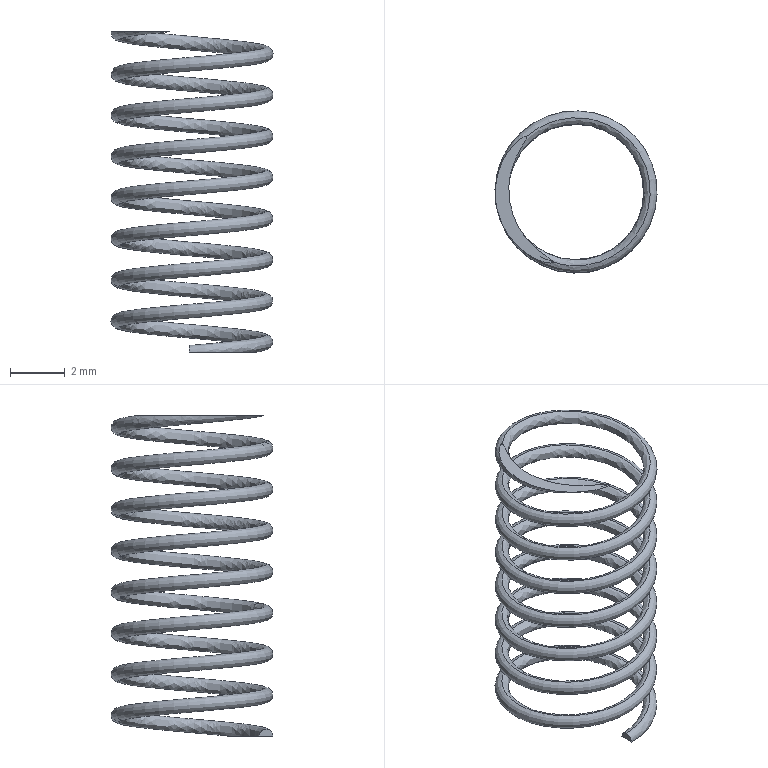Part | SolidWorks | features BaseBody 1 | 1 solid | 5 faces | box 5.908 x 5.904 x 11.688 mm | volume 28.098 mm3 | plane 3 | spline 2